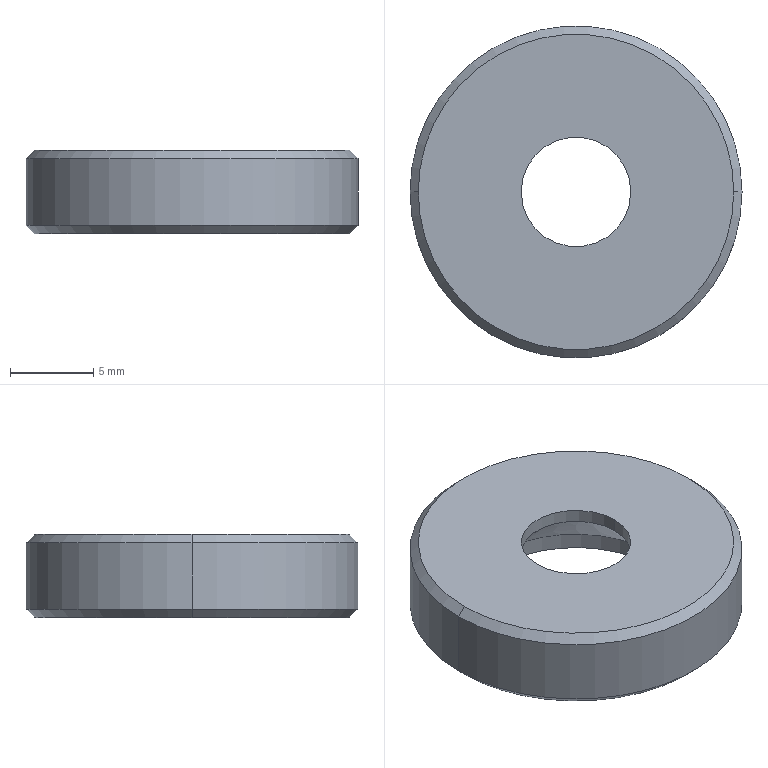Part | Creo | 1 solid | 14 faces | box 20 x 20 x 5 mm | volume 1145 mm3 | cone 6 | cylinder 6 | plane 2 | commonest cylinder face diameters 6.6 x2 13 x2 20 x2
STEP:
#1=CARTESIAN_POINT('',(0.,0.,0.));
#2=DIRECTION('',(0.,0.,1.));
#3=DIRECTION('',(1.,0.,0.));
#4=AXIS2_PLACEMENT_3D('',#1,#2,#3);
#5=CARTESIAN_POINT('',(55.5,35.,-260.5));
#6=VERTEX_POINT('',#5);
#7=CARTESIAN_POINT('',(74.5,35.,-260.5));
#8=VERTEX_POINT('',#7);
#9=CARTESIAN_POINT('',(65.,35.,-260.5));
#10=DIRECTION('',(0.,0.,-1.));
#11=DIRECTION('',(-1.,0.,0.));
#12=AXIS2_PLACEMENT_3D('',#9,#10,#11);
#13=CIRCLE('',#12,9.5);
#14=EDGE_CURVE('',#6,#8,#13,.T.);
#15=ORIENTED_EDGE('',*,*,#14,.F.);
#16=CARTESIAN_POINT('',(65.,35.,-260.5));
#17=DIRECTION('',(0.,0.,-1.));
#18=DIRECTION('',(1.,0.,0.));
#19=AXIS2_PLACEMENT_3D('',#16,#17,#18);
#20=CIRCLE('',#19,9.5);
#21=EDGE_CURVE('',#8,#6,#20,.T.);
#22=ORIENTED_EDGE('',*,*,#21,.F.);
#23=EDGE_LOOP('',(#15,#22));
#24=FACE_OUTER_BOUND('',#23,.F.);
#25=CARTESIAN_POINT('',(71.5,35.,-260.5));
#26=VERTEX_POINT('',#25);
#27=CARTESIAN_POINT('',(58.5,35.,-260.5));
#28=VERTEX_POINT('',#27);
#29=CARTESIAN_POINT('',(65.,35.,-260.5));
#30=DIRECTION('',(0.,0.,1.));
#31=DIRECTION('',(1.,0.,0.));
#32=AXIS2_PLACEMENT_3D('',#29,#30,#31);
#33=CIRCLE('',#32,6.5);
#34=EDGE_CURVE('',#26,#28,#33,.T.);
#35=ORIENTED_EDGE('',*,*,#34,.F.);
#36=CARTESIAN_POINT('',(65.,35.,-260.5));
#37=DIRECTION('',(0.,0.,1.));
#38=DIRECTION('',(-1.,0.,0.));
#39=AXIS2_PLACEMENT_3D('',#36,#37,#38);
#40=CIRCLE('',#39,6.5);
#41=EDGE_CURVE('',#28,#26,#40,.T.);
#42=ORIENTED_EDGE('',*,*,#41,.F.);
#43=EDGE_LOOP('',(#35,#42));
#44=FACE_BOUND('',#43,.F.);
#45=CARTESIAN_POINT('',(65.,35.,-260.5));
#46=DIRECTION('',(0.,0.,-1.));
#47=DIRECTION('',(-1.,0.,0.));
#48=AXIS2_PLACEMENT_3D('',#45,#46,#47);
#49=PLANE('',#48);
#50=ADVANCED_FACE('',(#24,#44),#49,.T.);
#51=CARTESIAN_POINT('',(55.,35.,-260.));
#52=VERTEX_POINT('',#51);
#53=CARTESIAN_POINT('',(75.,35.,-260.));
#54=VERTEX_POINT('',#53);
#55=CARTESIAN_POINT('',(65.,35.,-260.));
#56=DIRECTION('',(0.,0.,-1.));
#57=DIRECTION('',(-1.,0.,0.));
#58=AXIS2_PLACEMENT_3D('',#55,#56,#57);
#59=CIRCLE('',#58,10.);
#60=EDGE_CURVE('',#52,#54,#59,.T.);
#61=ORIENTED_EDGE('',*,*,#60,.F.);
#62=CARTESIAN_POINT('',(55.5,35.,-260.5));
#63=DIRECTION('',(-0.7071,0.,0.7071));
#64=VECTOR('',#63,0.7071);
#65=LINE('',#62,#64);
#66=EDGE_CURVE('',#6,#52,#65,.T.);
#67=ORIENTED_EDGE('',*,*,#66,.F.);
#68=ORIENTED_EDGE('',*,*,#14,.T.);
#69=CARTESIAN_POINT('',(74.5,35.,-260.5));
#70=DIRECTION('',(0.7071,0.,0.7071));
#71=VECTOR('',#70,0.7071);
#72=LINE('',#69,#71);
#73=EDGE_CURVE('',#8,#54,#72,.T.);
#74=ORIENTED_EDGE('',*,*,#73,.T.);
#75=EDGE_LOOP('',(#61,#67,#68,#74));
#76=FACE_OUTER_BOUND('',#75,.F.);
#77=CARTESIAN_POINT('',(65.,35.,-260.25));
#78=DIRECTION('',(0.,0.,1.));
#79=DIRECTION('',(1.,0.,0.));
#80=AXIS2_PLACEMENT_3D('',#77,#78,#79);
#81=CONICAL_SURFACE('',#80,9.75,45.);
#82=ADVANCED_FACE('',(#76),#81,.T.);
#83=CARTESIAN_POINT('',(75.,35.,-256.));
#84=VERTEX_POINT('',#83);
#85=CARTESIAN_POINT('',(55.,35.,-256.));
#86=VERTEX_POINT('',#85);
#87=CARTESIAN_POINT('',(65.,35.,-256.));
#88=DIRECTION('',(0.,0.,1.));
#89=DIRECTION('',(1.,0.,0.));
#90=AXIS2_PLACEMENT_3D('',#87,#88,#89);
#91=CIRCLE('',#90,10.);
#92=EDGE_CURVE('',#84,#86,#91,.T.);
#93=ORIENTED_EDGE('',*,*,#92,.T.);
#94=CARTESIAN_POINT('',(55.,35.,-260.));
#95=DIRECTION('',(0.,0.,1.));
#96=VECTOR('',#95,4.);
#97=LINE('',#94,#96);
#98=EDGE_CURVE('',#52,#86,#97,.T.);
#99=ORIENTED_EDGE('',*,*,#98,.F.);
#100=ORIENTED_EDGE('',*,*,#60,.T.);
#101=CARTESIAN_POINT('',(75.,35.,-260.));
#102=DIRECTION('',(0.,0.,1.));
#103=VECTOR('',#102,4.);
#104=LINE('',#101,#103);
#105=EDGE_CURVE('',#54,#84,#104,.T.);
#106=ORIENTED_EDGE('',*,*,#105,.T.);
#107=EDGE_LOOP('',(#93,#99,#100,#106));
#108=FACE_OUTER_BOUND('',#107,.F.);
#109=CARTESIAN_POINT('',(65.,35.,-260.5));
#110=DIRECTION('',(0.,0.,1.));
#111=DIRECTION('',(1.,0.,0.));
#112=AXIS2_PLACEMENT_3D('',#109,#110,#111);
#113=CYLINDRICAL_SURFACE('',#112,10.);
#114=ADVANCED_FACE('',(#108),#113,.T.);
#115=CARTESIAN_POINT('',(74.5,35.,-255.5));
#116=VERTEX_POINT('',#115);
#117=CARTESIAN_POINT('',(55.5,35.,-255.5));
#118=VERTEX_POINT('',#117);
#119=CARTESIAN_POINT('',(65.,35.,-255.5));
#120=DIRECTION('',(0.,0.,1.));
#121=DIRECTION('',(1.,0.,0.));
#122=AXIS2_PLACEMENT_3D('',#119,#120,#121);
#123=CIRCLE('',#122,9.5);
#124=EDGE_CURVE('',#116,#118,#123,.T.);
#125=ORIENTED_EDGE('',*,*,#124,.T.);
#126=CARTESIAN_POINT('',(55.5,35.,-255.5));
#127=DIRECTION('',(-0.7071,0.,-0.7071));
#128=VECTOR('',#127,0.7071);
#129=LINE('',#126,#128);
#130=EDGE_CURVE('',#118,#86,#129,.T.);
#131=ORIENTED_EDGE('',*,*,#130,.T.);
#132=ORIENTED_EDGE('',*,*,#92,.F.);
#133=CARTESIAN_POINT('',(74.5,35.,-255.5));
#134=DIRECTION('',(0.7071,0.,-0.7071));
#135=VECTOR('',#134,0.7071);
#136=LINE('',#133,#135);
#137=EDGE_CURVE('',#116,#84,#136,.T.);
#138=ORIENTED_EDGE('',*,*,#137,.F.);
#139=EDGE_LOOP('',(#125,#131,#132,#138));
#140=FACE_OUTER_BOUND('',#139,.F.);
#141=CARTESIAN_POINT('',(65.,35.,-255.75));
#142=DIRECTION('',(0.,0.,-1.));
#143=DIRECTION('',(-1.,0.,0.));
#144=AXIS2_PLACEMENT_3D('',#141,#142,#143);
#145=CONICAL_SURFACE('',#144,9.75,45.);
#146=ADVANCED_FACE('',(#140),#145,.T.);
#147=CARTESIAN_POINT('',(65.,35.,-255.5));
#148=DIRECTION('',(0.,0.,1.));
#149=DIRECTION('',(-1.,0.,0.));
#150=AXIS2_PLACEMENT_3D('',#147,#148,#149);
#151=CIRCLE('',#150,9.5);
#152=EDGE_CURVE('',#118,#116,#151,.T.);
#153=ORIENTED_EDGE('',*,*,#152,.F.);
#154=ORIENTED_EDGE('',*,*,#124,.F.);
#155=EDGE_LOOP('',(#153,#154));
#156=FACE_OUTER_BOUND('',#155,.F.);
#157=CARTESIAN_POINT('',(68.3,35.,-255.5));
#158=VERTEX_POINT('',#157);
#159=CARTESIAN_POINT('',(61.7,35.,-255.5));
#160=VERTEX_POINT('',#159);
#161=CARTESIAN_POINT('',(65.,35.,-255.5));
#162=DIRECTION('',(0.,0.,-1.));
#163=DIRECTION('',(1.,0.,0.));
#164=AXIS2_PLACEMENT_3D('',#161,#162,#163);
#165=CIRCLE('',#164,3.3);
#166=EDGE_CURVE('',#158,#160,#165,.T.);
#167=ORIENTED_EDGE('',*,*,#166,.F.);
#168=CARTESIAN_POINT('',(65.,35.,-255.5));
#169=DIRECTION('',(0.,0.,-1.));
#170=DIRECTION('',(-1.,0.,0.));
#171=AXIS2_PLACEMENT_3D('',#168,#169,#170);
#172=CIRCLE('',#171,3.3);
#173=EDGE_CURVE('',#160,#158,#172,.T.);
#174=ORIENTED_EDGE('',*,*,#173,.F.);
#175=EDGE_LOOP('',(#167,#174));
#176=FACE_BOUND('',#175,.F.);
#177=CARTESIAN_POINT('',(65.,35.,-255.5));
#178=DIRECTION('',(0.,0.,-1.));
#179=DIRECTION('',(-1.,0.,0.));
#180=AXIS2_PLACEMENT_3D('',#177,#178,#179);
#181=PLANE('',#180);
#182=ADVANCED_FACE('',(#156,#176),#181,.F.);
#183=ORIENTED_EDGE('',*,*,#152,.T.);
#184=ORIENTED_EDGE('',*,*,#137,.T.);
#185=CARTESIAN_POINT('',(65.,35.,-256.));
#186=DIRECTION('',(0.,0.,1.));
#187=DIRECTION('',(-1.,0.,0.));
#188=AXIS2_PLACEMENT_3D('',#185,#186,#187);
#189=CIRCLE('',#188,10.);
#190=EDGE_CURVE('',#86,#84,#189,.T.);
#191=ORIENTED_EDGE('',*,*,#190,.F.);
#192=ORIENTED_EDGE('',*,*,#130,.F.);
#193=EDGE_LOOP('',(#183,#184,#191,#192));
#194=FACE_OUTER_BOUND('',#193,.F.);
#195=CARTESIAN_POINT('',(65.,35.,-255.75));
#196=DIRECTION('',(0.,0.,-1.));
#197=DIRECTION('',(-1.,0.,0.));
#198=AXIS2_PLACEMENT_3D('',#195,#196,#197);
#199=CONICAL_SURFACE('',#198,9.75,45.);
#200=ADVANCED_FACE('',(#194),#199,.T.);
#201=ORIENTED_EDGE('',*,*,#190,.T.);
#202=ORIENTED_EDGE('',*,*,#105,.F.);
#203=CARTESIAN_POINT('',(65.,35.,-260.));
#204=DIRECTION('',(0.,0.,-1.));
#205=DIRECTION('',(1.,0.,0.));
#206=AXIS2_PLACEMENT_3D('',#203,#204,#205);
#207=CIRCLE('',#206,10.);
#208=EDGE_CURVE('',#54,#52,#207,.T.);
#209=ORIENTED_EDGE('',*,*,#208,.T.);
#210=ORIENTED_EDGE('',*,*,#98,.T.);
#211=EDGE_LOOP('',(#201,#202,#209,#210));
#212=FACE_OUTER_BOUND('',#211,.F.);
#213=CARTESIAN_POINT('',(65.,35.,-260.5));
#214=DIRECTION('',(0.,0.,1.));
#215=DIRECTION('',(1.,0.,0.));
#216=AXIS2_PLACEMENT_3D('',#213,#214,#215);
#217=CYLINDRICAL_SURFACE('',#216,10.);
#218=ADVANCED_FACE('',(#212),#217,.T.);
#219=ORIENTED_EDGE('',*,*,#208,.F.);
#220=ORIENTED_EDGE('',*,*,#73,.F.);
#221=ORIENTED_EDGE('',*,*,#21,.T.);
#222=ORIENTED_EDGE('',*,*,#66,.T.);
#223=EDGE_LOOP('',(#219,#220,#221,#222));
#224=FACE_OUTER_BOUND('',#223,.F.);
#225=CARTESIAN_POINT('',(65.,35.,-260.25));
#226=DIRECTION('',(0.,0.,1.));
#227=DIRECTION('',(1.,0.,0.));
#228=AXIS2_PLACEMENT_3D('',#225,#226,#227);
#229=CONICAL_SURFACE('',#228,9.75,45.);
#230=ADVANCED_FACE('',(#224),#229,.T.);
#231=CARTESIAN_POINT('',(61.7,35.,-256.3));
#232=VERTEX_POINT('',#231);
#233=CARTESIAN_POINT('',(68.3,35.,-256.3));
#234=VERTEX_POINT('',#233);
#235=CARTESIAN_POINT('',(65.,35.,-256.3));
#236=DIRECTION('',(0.,0.,1.));
#237=DIRECTION('',(-1.,0.,0.));
#238=AXIS2_PLACEMENT_3D('',#235,#236,#237);
#239=CIRCLE('',#238,3.3);
#240=EDGE_CURVE('',#232,#234,#239,.T.);
#241=ORIENTED_EDGE('',*,*,#240,.T.);
#242=CARTESIAN_POINT('',(68.3,35.,-256.3));
#243=DIRECTION('',(0.,0.,1.));
#244=VECTOR('',#243,0.8);
#245=LINE('',#242,#244);
#246=EDGE_CURVE('',#234,#158,#245,.T.);
#247=ORIENTED_EDGE('',*,*,#246,.T.);
#248=ORIENTED_EDGE('',*,*,#166,.T.);
#249=CARTESIAN_POINT('',(61.7,35.,-256.3));
#250=DIRECTION('',(0.,0.,1.));
#251=VECTOR('',#250,0.8);
#252=LINE('',#249,#251);
#253=EDGE_CURVE('',#232,#160,#252,.T.);
#254=ORIENTED_EDGE('',*,*,#253,.F.);
#255=EDGE_LOOP('',(#241,#247,#248,#254));
#256=FACE_OUTER_BOUND('',#255,.F.);
#257=CARTESIAN_POINT('',(65.,35.,-255.5));
#258=DIRECTION('',(0.,0.,1.));
#259=DIRECTION('',(1.,0.,0.));
#260=AXIS2_PLACEMENT_3D('',#257,#258,#259);
#261=CYLINDRICAL_SURFACE('',#260,3.3);
#262=ADVANCED_FACE('',(#256),#261,.F.);
#263=CARTESIAN_POINT('',(71.5,35.,-259.5));
#264=VERTEX_POINT('',#263);
#265=CARTESIAN_POINT('',(58.5,35.,-259.5));
#266=VERTEX_POINT('',#265);
#267=CARTESIAN_POINT('',(65.,35.,-259.5));
#268=DIRECTION('',(0.,0.,-1.));
#269=DIRECTION('',(1.,0.,0.));
#270=AXIS2_PLACEMENT_3D('',#267,#268,#269);
#271=CIRCLE('',#270,6.5);
#272=EDGE_CURVE('',#264,#266,#271,.T.);
#273=ORIENTED_EDGE('',*,*,#272,.F.);
#274=CARTESIAN_POINT('',(68.3,35.,-256.3));
#275=DIRECTION('',(0.7071,0.,-0.7071));
#276=VECTOR('',#275,4.525);
#277=LINE('',#274,#276);
#278=EDGE_CURVE('',#234,#264,#277,.T.);
#279=ORIENTED_EDGE('',*,*,#278,.F.);
#280=ORIENTED_EDGE('',*,*,#240,.F.);
#281=CARTESIAN_POINT('',(61.7,35.,-256.3));
#282=DIRECTION('',(-0.7071,0.,-0.7071));
#283=VECTOR('',#282,4.525);
#284=LINE('',#281,#283);
#285=EDGE_CURVE('',#232,#266,#284,.T.);
#286=ORIENTED_EDGE('',*,*,#285,.T.);
#287=EDGE_LOOP('',(#273,#279,#280,#286));
#288=FACE_OUTER_BOUND('',#287,.F.);
#289=CARTESIAN_POINT('',(65.,35.,-257.9));
#290=DIRECTION('',(0.,0.,-1.));
#291=DIRECTION('',(-1.,0.,0.));
#292=AXIS2_PLACEMENT_3D('',#289,#290,#291);
#293=CONICAL_SURFACE('',#292,4.9,45.);
#294=ADVANCED_FACE('',(#288),#293,.F.);
#295=ORIENTED_EDGE('',*,*,#41,.T.);
#296=CARTESIAN_POINT('',(71.5,35.,-260.5));
#297=DIRECTION('',(0.,0.,1.));
#298=VECTOR('',#297,1.);
#299=LINE('',#296,#298);
#300=EDGE_CURVE('',#26,#264,#299,.T.);
#301=ORIENTED_EDGE('',*,*,#300,.T.);
#302=ORIENTED_EDGE('',*,*,#272,.T.);
#303=CARTESIAN_POINT('',(58.5,35.,-260.5));
#304=DIRECTION('',(0.,0.,1.));
#305=VECTOR('',#304,1.);
#306=LINE('',#303,#305);
#307=EDGE_CURVE('',#28,#266,#306,.T.);
#308=ORIENTED_EDGE('',*,*,#307,.F.);
#309=EDGE_LOOP('',(#295,#301,#302,#308));
#310=FACE_OUTER_BOUND('',#309,.F.);
#311=CARTESIAN_POINT('',(65.,35.,-255.5));
#312=DIRECTION('',(0.,0.,1.));
#313=DIRECTION('',(1.,0.,0.));
#314=AXIS2_PLACEMENT_3D('',#311,#312,#313);
#315=CYLINDRICAL_SURFACE('',#314,6.5);
#316=ADVANCED_FACE('',(#310),#315,.F.);
#317=ORIENTED_EDGE('',*,*,#34,.T.);
#318=ORIENTED_EDGE('',*,*,#307,.T.);
#319=CARTESIAN_POINT('',(65.,35.,-259.5));
#320=DIRECTION('',(0.,0.,-1.));
#321=DIRECTION('',(-1.,0.,0.));
#322=AXIS2_PLACEMENT_3D('',#319,#320,#321);
#323=CIRCLE('',#322,6.5);
#324=EDGE_CURVE('',#266,#264,#323,.T.);
#325=ORIENTED_EDGE('',*,*,#324,.T.);
#326=ORIENTED_EDGE('',*,*,#300,.F.);
#327=EDGE_LOOP('',(#317,#318,#325,#326));
#328=FACE_OUTER_BOUND('',#327,.F.);
#329=CARTESIAN_POINT('',(65.,35.,-255.5));
#330=DIRECTION('',(0.,0.,1.));
#331=DIRECTION('',(1.,0.,0.));
#332=AXIS2_PLACEMENT_3D('',#329,#330,#331);
#333=CYLINDRICAL_SURFACE('',#332,6.5);
#334=ADVANCED_FACE('',(#328),#333,.F.);
#335=ORIENTED_EDGE('',*,*,#324,.F.);
#336=ORIENTED_EDGE('',*,*,#285,.F.);
#337=CARTESIAN_POINT('',(65.,35.,-256.3));
#338=DIRECTION('',(0.,0.,1.));
#339=DIRECTION('',(1.,0.,0.));
#340=AXIS2_PLACEMENT_3D('',#337,#338,#339);
#341=CIRCLE('',#340,3.3);
#342=EDGE_CURVE('',#234,#232,#341,.T.);
#343=ORIENTED_EDGE('',*,*,#342,.F.);
#344=ORIENTED_EDGE('',*,*,#278,.T.);
#345=EDGE_LOOP('',(#335,#336,#343,#344));
#346=FACE_OUTER_BOUND('',#345,.F.);
#347=CARTESIAN_POINT('',(65.,35.,-257.9));
#348=DIRECTION('',(0.,0.,-1.));
#349=DIRECTION('',(-1.,0.,0.));
#350=AXIS2_PLACEMENT_3D('',#347,#348,#349);
#351=CONICAL_SURFACE('',#350,4.9,45.);
#352=ADVANCED_FACE('',(#346),#351,.F.);
#353=ORIENTED_EDGE('',*,*,#342,.T.);
#354=ORIENTED_EDGE('',*,*,#253,.T.);
#355=ORIENTED_EDGE('',*,*,#173,.T.);
#356=ORIENTED_EDGE('',*,*,#246,.F.);
#357=EDGE_LOOP('',(#353,#354,#355,#356));
#358=FACE_OUTER_BOUND('',#357,.F.);
#359=CARTESIAN_POINT('',(65.,35.,-255.5));
#360=DIRECTION('',(0.,0.,1.));
#361=DIRECTION('',(1.,0.,0.));
#362=AXIS2_PLACEMENT_3D('',#359,#360,#361);
#363=CYLINDRICAL_SURFACE('',#362,3.3);
#364=ADVANCED_FACE('',(#358),#363,.F.);
#365=CLOSED_SHELL('',(#50,#82,#114,#146,#182,#200,#218,#230,#262,#294,#316,#334,#352,#364));
#366=MANIFOLD_SOLID_BREP('',#365);
#367=(LENGTH_UNIT()NAMED_UNIT(*)SI_UNIT(.MILLI.,.METRE.));
#368=UNCERTAINTY_MEASURE_WITH_UNIT(LENGTH_MEASURE(0.002872),#367,'','');
#369=(NAMED_UNIT(*)PLANE_ANGLE_UNIT()SI_UNIT($,.RADIAN.));
#370=PLANE_ANGLE_MEASURE_WITH_UNIT(PLANE_ANGLE_MEASURE(0.01745),#369);
#371=(CONVERSION_BASED_UNIT('DEGREE',#370)NAMED_UNIT(*)PLANE_ANGLE_UNIT());
#372=(NAMED_UNIT(*)SI_UNIT($,.STERADIAN.)SOLID_ANGLE_UNIT());
#373=(GEOMETRIC_REPRESENTATION_CONTEXT(3)GLOBAL_UNCERTAINTY_ASSIGNED_CONTEXT((#368))GLOBAL_UNIT_ASSIGNED_CONTEXT((#367,#371,#372))REPRESENTATION_CONTEXT('',''));
#374=ADVANCED_BREP_SHAPE_REPRESENTATION('',(#4,#366),#373);